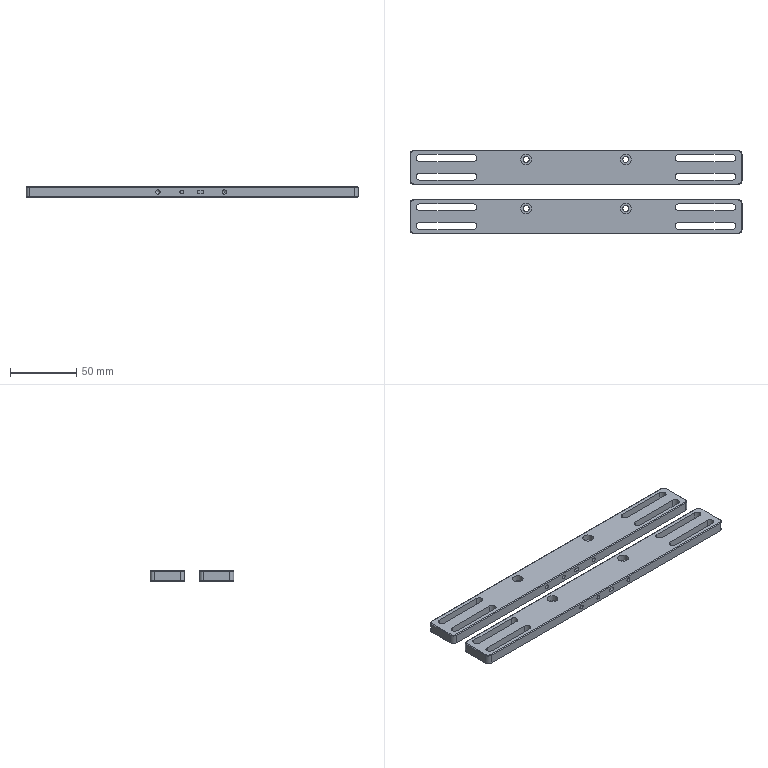NC program | NX | posted with a generic post | part box 250 x 63 x 8 mm
Lines 1 to 29 of 4328:
N10 G17 G21 G94 G90
(DRILLING_COPY_1_COPY_1_COPY , TOOL : D6A45)
N12 T22 M6
N14 G54
N16 G17 G0 G90 X-24.351 Y0. B0. C0. S5000 M3
N18 G43 Z30. H22
N20 G94 G81 G98 Z-1. F250. R3.
N22 X-5.601
N24 X7.649
N26 X25.649
N28 G80
N30 G0 X25.649 Y0. Z30.
N32 M5
(DRILLING_COPY_1_COPY_COPY_COPY_COPY_1_COPY , TOOL : 3.3ZT)
N34 T19 M6
N36 G54
N38 G17 G0 G90 X-24.351 Y0. B0. C0. S2000 M3
N40 G43 Z30. H19
N42 G94 G83 G98 Z-15.974 F150. Q2. R3.
N44 X25.649
N46 G80
N48 G0 X25.649 Y0. Z30.
N50 M5